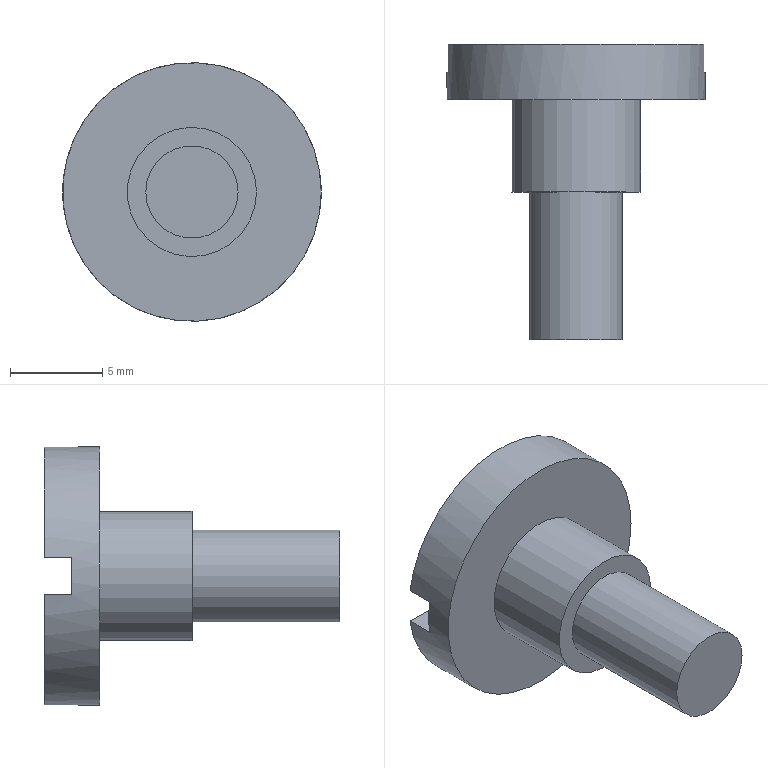Part | STEP file | 2-06.5 | 1 solid | 11 faces | box 14 x 16 x 14 mm | volume 769.46 mm3 | plane 8 | cylinder 3 | commonest cylinder face diameters 5 x1 7 x1 14 x1
STEP:
#1=CARTESIAN_POINT('',(0.,0.,0.));
#2=DIRECTION('',(0.,0.,1.));
#3=DIRECTION('',(1.,0.,0.));
#4=AXIS2_PLACEMENT_3D('',#1,#2,#3);
#5=CARTESIAN_POINT('',(3.5,0.,0.));
#6=VERTEX_POINT('',#5);
#7=CARTESIAN_POINT('',(0.,0.,0.));
#8=DIRECTION('',(0.,-1.,0.));
#9=DIRECTION('',(1.,0.,0.));
#10=AXIS2_PLACEMENT_3D('',#7,#8,#9);
#11=CIRCLE('',#10,3.5);
#12=CARTESIAN_POINT('',(0.,0.,0.));
#13=DIRECTION('',(0.,-1.,0.));
#14=DIRECTION('',(1.,0.,0.));
#15=AXIS2_PLACEMENT_3D('',#12,#13,#14);
#16=CYLINDRICAL_SURFACE('',#15,3.5);
#17=CARTESIAN_POINT('',(0.,0.));
#18=DIRECTION('',(1.,0.));
#19=VECTOR('',#18,1.);
#20=LINE('',#17,#19);
#21=(GEOMETRIC_REPRESENTATION_CONTEXT(2)PARAMETRIC_REPRESENTATION_CONTEXT()REPRESENTATION_CONTEXT('',''));
#22=DEFINITIONAL_REPRESENTATION('',(#20),#21);
#23=PCURVE('',#16,#22);
#24=CARTESIAN_POINT('',(-1.876,0.,0.));
#25=DIRECTION('',(0.,-1.,0.));
#26=DIRECTION('',(1.,0.,0.));
#27=AXIS2_PLACEMENT_3D('',#24,#25,#26);
#28=PLANE('',#27);
#29=CARTESIAN_POINT('',(1.876,0.));
#30=DIRECTION('',(1.,0.));
#31=AXIS2_PLACEMENT_2D('',#29,#30);
#32=CIRCLE('',#31,3.5);
#33=(GEOMETRIC_REPRESENTATION_CONTEXT(2)PARAMETRIC_REPRESENTATION_CONTEXT()REPRESENTATION_CONTEXT('',''));
#34=DEFINITIONAL_REPRESENTATION('',(#32),#33);
#35=PCURVE('',#28,#34);
#36=SURFACE_CURVE('',#11,(#23,#35),.PCURVE_S1.);
#37=EDGE_CURVE('',#6,#6,#36,.T.);
#38=ORIENTED_EDGE('',*,*,#37,.T.);
#39=CARTESIAN_POINT('',(3.5,-5.,0.));
#40=VERTEX_POINT('',#39);
#41=CARTESIAN_POINT('',(3.5,0.,0.));
#42=DIRECTION('',(0.,-1.,0.));
#43=VECTOR('',#42,1.);
#44=LINE('',#41,#43);
#45=CARTESIAN_POINT('',(6.283,0.));
#46=DIRECTION('',(0.,1.));
#47=VECTOR('',#46,1.);
#48=LINE('',#45,#47);
#49=(GEOMETRIC_REPRESENTATION_CONTEXT(2)PARAMETRIC_REPRESENTATION_CONTEXT()REPRESENTATION_CONTEXT('',''));
#50=DEFINITIONAL_REPRESENTATION('',(#48),#49);
#51=PCURVE('',#16,#50);
#52=CARTESIAN_POINT('',(0.,0.));
#53=DIRECTION('',(0.,1.));
#54=VECTOR('',#53,1.);
#55=LINE('',#52,#54);
#56=(GEOMETRIC_REPRESENTATION_CONTEXT(2)PARAMETRIC_REPRESENTATION_CONTEXT()REPRESENTATION_CONTEXT('',''));
#57=DEFINITIONAL_REPRESENTATION('',(#55),#56);
#58=PCURVE('',#16,#57);
#59=SEAM_CURVE('',#44,(#51,#58),.PCURVE_S1.);
#60=EDGE_CURVE('',#6,#40,#59,.T.);
#61=ORIENTED_EDGE('',*,*,#60,.T.);
#62=CARTESIAN_POINT('',(0.,-5.,0.));
#63=DIRECTION('',(0.,-1.,0.));
#64=DIRECTION('',(1.,0.,0.));
#65=AXIS2_PLACEMENT_3D('',#62,#63,#64);
#66=CIRCLE('',#65,3.5);
#67=CARTESIAN_POINT('',(0.,5.));
#68=DIRECTION('',(1.,0.));
#69=VECTOR('',#68,1.);
#70=LINE('',#67,#69);
#71=(GEOMETRIC_REPRESENTATION_CONTEXT(2)PARAMETRIC_REPRESENTATION_CONTEXT()REPRESENTATION_CONTEXT('',''));
#72=DEFINITIONAL_REPRESENTATION('',(#70),#71);
#73=PCURVE('',#16,#72);
#74=CARTESIAN_POINT('',(-0.9378,-5.,0.));
#75=DIRECTION('',(0.,-1.,0.));
#76=DIRECTION('',(1.,0.,0.));
#77=AXIS2_PLACEMENT_3D('',#74,#75,#76);
#78=PLANE('',#77);
#79=CARTESIAN_POINT('',(0.9378,0.));
#80=DIRECTION('',(1.,0.));
#81=AXIS2_PLACEMENT_2D('',#79,#80);
#82=CIRCLE('',#81,3.5);
#83=(GEOMETRIC_REPRESENTATION_CONTEXT(2)PARAMETRIC_REPRESENTATION_CONTEXT()REPRESENTATION_CONTEXT('',''));
#84=DEFINITIONAL_REPRESENTATION('',(#82),#83);
#85=PCURVE('',#78,#84);
#86=SURFACE_CURVE('',#66,(#73,#85),.PCURVE_S1.);
#87=EDGE_CURVE('',#40,#40,#86,.T.);
#88=ORIENTED_EDGE('',*,*,#87,.F.);
#89=ORIENTED_EDGE('',*,*,#60,.F.);
#90=EDGE_LOOP('',(#38,#61,#88,#89));
#91=FACE_BOUND('',#90,.T.);
#92=ADVANCED_FACE('',(#91),#16,.T.);
#93=CARTESIAN_POINT('',(7.,0.,0.));
#94=VERTEX_POINT('',#93);
#95=CARTESIAN_POINT('',(0.,0.,0.));
#96=DIRECTION('',(0.,-1.,0.));
#97=DIRECTION('',(1.,0.,0.));
#98=AXIS2_PLACEMENT_3D('',#95,#96,#97);
#99=CIRCLE('',#98,7.);
#100=CARTESIAN_POINT('',(1.876,0.));
#101=DIRECTION('',(1.,0.));
#102=AXIS2_PLACEMENT_2D('',#100,#101);
#103=CIRCLE('',#102,7.);
#104=(GEOMETRIC_REPRESENTATION_CONTEXT(2)PARAMETRIC_REPRESENTATION_CONTEXT()REPRESENTATION_CONTEXT('',''));
#105=DEFINITIONAL_REPRESENTATION('',(#103),#104);
#106=PCURVE('',#28,#105);
#107=CARTESIAN_POINT('',(0.,0.,0.));
#108=DIRECTION('',(0.,1.,0.));
#109=DIRECTION('',(1.,0.,0.));
#110=AXIS2_PLACEMENT_3D('',#107,#108,#109);
#111=CYLINDRICAL_SURFACE('',#110,7.);
#112=CARTESIAN_POINT('',(6.283,0.));
#113=DIRECTION('',(-1.,0.));
#114=VECTOR('',#113,1.);
#115=LINE('',#112,#114);
#116=(GEOMETRIC_REPRESENTATION_CONTEXT(2)PARAMETRIC_REPRESENTATION_CONTEXT()REPRESENTATION_CONTEXT('',''));
#117=DEFINITIONAL_REPRESENTATION('',(#115),#116);
#118=PCURVE('',#111,#117);
#119=SURFACE_CURVE('',#99,(#106,#118),.PCURVE_S1.);
#120=EDGE_CURVE('',#94,#94,#119,.T.);
#121=ORIENTED_EDGE('',*,*,#120,.T.);
#122=EDGE_LOOP('',(#121));
#123=FACE_BOUND('',#122,.T.);
#124=ORIENTED_EDGE('',*,*,#37,.F.);
#125=EDGE_LOOP('',(#124));
#126=FACE_BOUND('',#125,.T.);
#127=ADVANCED_FACE('',(#123,#126),#28,.T.);
#128=ORIENTED_EDGE('',*,*,#87,.T.);
#129=EDGE_LOOP('',(#128));
#130=FACE_BOUND('',#129,.T.);
#131=CARTESIAN_POINT('',(2.5,-5.,0.));
#132=VERTEX_POINT('',#131);
#133=CARTESIAN_POINT('',(0.,-5.,0.));
#134=DIRECTION('',(0.,-1.,0.));
#135=DIRECTION('',(1.,0.,0.));
#136=AXIS2_PLACEMENT_3D('',#133,#134,#135);
#137=CIRCLE('',#136,2.5);
#138=CARTESIAN_POINT('',(0.9378,0.));
#139=DIRECTION('',(1.,0.));
#140=AXIS2_PLACEMENT_2D('',#138,#139);
#141=CIRCLE('',#140,2.5);
#142=(GEOMETRIC_REPRESENTATION_CONTEXT(2)PARAMETRIC_REPRESENTATION_CONTEXT()REPRESENTATION_CONTEXT('',''));
#143=DEFINITIONAL_REPRESENTATION('',(#141),#142);
#144=PCURVE('',#78,#143);
#145=CARTESIAN_POINT('',(0.,-5.,0.));
#146=DIRECTION('',(0.,-1.,0.));
#147=DIRECTION('',(1.,0.,0.));
#148=AXIS2_PLACEMENT_3D('',#145,#146,#147);
#149=CYLINDRICAL_SURFACE('',#148,2.5);
#150=CARTESIAN_POINT('',(0.,0.));
#151=DIRECTION('',(1.,0.));
#152=VECTOR('',#151,1.);
#153=LINE('',#150,#152);
#154=(GEOMETRIC_REPRESENTATION_CONTEXT(2)PARAMETRIC_REPRESENTATION_CONTEXT()REPRESENTATION_CONTEXT('',''));
#155=DEFINITIONAL_REPRESENTATION('',(#153),#154);
#156=PCURVE('',#149,#155);
#157=SURFACE_CURVE('',#137,(#144,#156),.PCURVE_S1.);
#158=EDGE_CURVE('',#132,#132,#157,.T.);
#159=ORIENTED_EDGE('',*,*,#158,.F.);
#160=EDGE_LOOP('',(#159));
#161=FACE_BOUND('',#160,.T.);
#162=ADVANCED_FACE('',(#130,#161),#78,.T.);
#163=ORIENTED_EDGE('',*,*,#158,.T.);
#164=CARTESIAN_POINT('',(2.5,-13.,0.));
#165=VERTEX_POINT('',#164);
#166=CARTESIAN_POINT('',(2.5,-5.,0.));
#167=DIRECTION('',(0.,-1.,0.));
#168=VECTOR('',#167,1.);
#169=LINE('',#166,#168);
#170=CARTESIAN_POINT('',(6.283,0.));
#171=DIRECTION('',(0.,1.));
#172=VECTOR('',#171,1.);
#173=LINE('',#170,#172);
#174=(GEOMETRIC_REPRESENTATION_CONTEXT(2)PARAMETRIC_REPRESENTATION_CONTEXT()REPRESENTATION_CONTEXT('',''));
#175=DEFINITIONAL_REPRESENTATION('',(#173),#174);
#176=PCURVE('',#149,#175);
#177=CARTESIAN_POINT('',(0.,0.));
#178=DIRECTION('',(0.,1.));
#179=VECTOR('',#178,1.);
#180=LINE('',#177,#179);
#181=(GEOMETRIC_REPRESENTATION_CONTEXT(2)PARAMETRIC_REPRESENTATION_CONTEXT()REPRESENTATION_CONTEXT('',''));
#182=DEFINITIONAL_REPRESENTATION('',(#180),#181);
#183=PCURVE('',#149,#182);
#184=SEAM_CURVE('',#169,(#176,#183),.PCURVE_S1.);
#185=EDGE_CURVE('',#132,#165,#184,.T.);
#186=ORIENTED_EDGE('',*,*,#185,.T.);
#187=CARTESIAN_POINT('',(0.,-13.,0.));
#188=DIRECTION('',(0.,-1.,0.));
#189=DIRECTION('',(1.,0.,0.));
#190=AXIS2_PLACEMENT_3D('',#187,#188,#189);
#191=CIRCLE('',#190,2.5);
#192=CARTESIAN_POINT('',(0.,8.));
#193=DIRECTION('',(1.,0.));
#194=VECTOR('',#193,1.);
#195=LINE('',#192,#194);
#196=(GEOMETRIC_REPRESENTATION_CONTEXT(2)PARAMETRIC_REPRESENTATION_CONTEXT()REPRESENTATION_CONTEXT('',''));
#197=DEFINITIONAL_REPRESENTATION('',(#195),#196);
#198=PCURVE('',#149,#197);
#199=CARTESIAN_POINT('',(-0.6699,-13.,0.));
#200=DIRECTION('',(0.,-1.,0.));
#201=DIRECTION('',(1.,0.,0.));
#202=AXIS2_PLACEMENT_3D('',#199,#200,#201);
#203=PLANE('',#202);
#204=CARTESIAN_POINT('',(0.6699,0.));
#205=DIRECTION('',(1.,0.));
#206=AXIS2_PLACEMENT_2D('',#204,#205);
#207=CIRCLE('',#206,2.5);
#208=(GEOMETRIC_REPRESENTATION_CONTEXT(2)PARAMETRIC_REPRESENTATION_CONTEXT()REPRESENTATION_CONTEXT('',''));
#209=DEFINITIONAL_REPRESENTATION('',(#207),#208);
#210=PCURVE('',#203,#209);
#211=SURFACE_CURVE('',#191,(#198,#210),.PCURVE_S1.);
#212=EDGE_CURVE('',#165,#165,#211,.T.);
#213=ORIENTED_EDGE('',*,*,#212,.F.);
#214=ORIENTED_EDGE('',*,*,#185,.F.);
#215=EDGE_LOOP('',(#163,#186,#213,#214));
#216=FACE_BOUND('',#215,.T.);
#217=ADVANCED_FACE('',(#216),#149,.T.);
#218=ORIENTED_EDGE('',*,*,#212,.T.);
#219=EDGE_LOOP('',(#218));
#220=FACE_BOUND('',#219,.T.);
#221=ADVANCED_FACE('',(#220),#203,.T.);
#222=CARTESIAN_POINT('',(7.,1.5,0.));
#223=VERTEX_POINT('',#222);
#224=CARTESIAN_POINT('',(7.,0.,0.));
#225=DIRECTION('',(0.,1.,0.));
#226=VECTOR('',#225,1.);
#227=LINE('',#224,#226);
#228=CARTESIAN_POINT('',(6.283,0.));
#229=DIRECTION('',(0.,1.));
#230=VECTOR('',#229,1.);
#231=LINE('',#228,#230);
#232=(GEOMETRIC_REPRESENTATION_CONTEXT(2)PARAMETRIC_REPRESENTATION_CONTEXT()REPRESENTATION_CONTEXT('',''));
#233=DEFINITIONAL_REPRESENTATION('',(#231),#232);
#234=PCURVE('',#111,#233);
#235=CARTESIAN_POINT('',(0.,0.));
#236=DIRECTION('',(0.,1.));
#237=VECTOR('',#236,1.);
#238=LINE('',#235,#237);
#239=(GEOMETRIC_REPRESENTATION_CONTEXT(2)PARAMETRIC_REPRESENTATION_CONTEXT()REPRESENTATION_CONTEXT('',''));
#240=DEFINITIONAL_REPRESENTATION('',(#238),#239);
#241=PCURVE('',#111,#240);
#242=SEAM_CURVE('',#227,(#234,#241),.PCURVE_S1.);
#243=EDGE_CURVE('',#94,#223,#242,.T.);
#244=ORIENTED_EDGE('',*,*,#243,.T.);
#245=CARTESIAN_POINT('',(6.928,1.5,1.));
#246=VERTEX_POINT('',#245);
#247=CARTESIAN_POINT('',(0.,1.5,0.));
#248=DIRECTION('',(0.,1.,0.));
#249=DIRECTION('',(0.9897,0.,0.1429));
#250=AXIS2_PLACEMENT_3D('',#247,#248,#249);
#251=CIRCLE('',#250,7.);
#252=CARTESIAN_POINT('',(6.14,1.5));
#253=DIRECTION('',(1.,0.));
#254=VECTOR('',#253,1.);
#255=LINE('',#252,#254);
#256=(GEOMETRIC_REPRESENTATION_CONTEXT(2)PARAMETRIC_REPRESENTATION_CONTEXT()REPRESENTATION_CONTEXT('',''));
#257=DEFINITIONAL_REPRESENTATION('',(#255),#256);
#258=PCURVE('',#111,#257);
#259=CARTESIAN_POINT('',(0.,1.5,0.));
#260=DIRECTION('',(0.,-1.,0.));
#261=DIRECTION('',(0.,0.,-1.));
#262=AXIS2_PLACEMENT_3D('',#259,#260,#261);
#263=PLANE('',#262);
#264=CARTESIAN_POINT('',(-1.,6.928));
#265=CARTESIAN_POINT('',(11.,8.66));
#266=CARTESIAN_POINT('',(6.5,-2.598));
#267=CARTESIAN_POINT('',(2.,-13.856));
#268=CARTESIAN_POINT('',(-5.5,-4.33));
#269=CARTESIAN_POINT('',(-13.,5.196));
#270=CARTESIAN_POINT('',(-1.,6.928));
#271=(BOUNDED_CURVE()B_SPLINE_CURVE(2,(#264,#265,#266,#267,#268,#269,#270),.UNSPECIFIED.,.T.,.F.)B_SPLINE_CURVE_WITH_KNOTS((1,2,2,2,2,1),(-2.094,0.,2.094,4.189,6.283,8.378),.UNSPECIFIED.)CURVE()GEOMETRIC_REPRESENTATION_ITEM()RATIONAL_B_SPLINE_CURVE((1.,0.5,1.,0.5,1.,0.5,1.))REPRESENTATION_ITEM(''));
#272=(GEOMETRIC_REPRESENTATION_CONTEXT(2)PARAMETRIC_REPRESENTATION_CONTEXT()REPRESENTATION_CONTEXT('',''));
#273=DEFINITIONAL_REPRESENTATION('',(#271),#272);
#274=PCURVE('',#263,#273);
#275=SURFACE_CURVE('',#251,(#258,#274),.PCURVE_S1.);
#276=EDGE_CURVE('',#246,#223,#275,.T.);
#277=ORIENTED_EDGE('',*,*,#276,.F.);
#278=CARTESIAN_POINT('',(6.928,3.,1.));
#279=VERTEX_POINT('',#278);
#280=CARTESIAN_POINT('',(6.928,3.,1.));
#281=DIRECTION('',(0.,-1.,0.));
#282=VECTOR('',#281,1.);
#283=LINE('',#280,#282);
#284=CARTESIAN_POINT('',(6.14,3.));
#285=DIRECTION('',(0.,-1.));
#286=VECTOR('',#285,1.);
#287=LINE('',#284,#286);
#288=(GEOMETRIC_REPRESENTATION_CONTEXT(2)PARAMETRIC_REPRESENTATION_CONTEXT()REPRESENTATION_CONTEXT('',''));
#289=DEFINITIONAL_REPRESENTATION('',(#287),#288);
#290=PCURVE('',#111,#289);
#291=CARTESIAN_POINT('',(0.,3.,1.));
#292=DIRECTION('',(0.,0.,1.));
#293=DIRECTION('',(0.,-1.,0.));
#294=AXIS2_PLACEMENT_3D('',#291,#292,#293);
#295=PLANE('',#294);
#296=CARTESIAN_POINT('',(0.,6.928));
#297=DIRECTION('',(1.,0.));
#298=VECTOR('',#297,1.);
#299=LINE('',#296,#298);
#300=(GEOMETRIC_REPRESENTATION_CONTEXT(2)PARAMETRIC_REPRESENTATION_CONTEXT()REPRESENTATION_CONTEXT('',''));
#301=DEFINITIONAL_REPRESENTATION('',(#299),#300);
#302=PCURVE('',#295,#301);
#303=SURFACE_CURVE('',#283,(#290,#302),.PCURVE_S1.);
#304=EDGE_CURVE('',#279,#246,#303,.T.);
#305=ORIENTED_EDGE('',*,*,#304,.F.);
#306=CARTESIAN_POINT('',(-6.928,3.,1.));
#307=VERTEX_POINT('',#306);
#308=CARTESIAN_POINT('',(0.,3.,0.));
#309=DIRECTION('',(0.,-1.,0.));
#310=DIRECTION('',(0.9897,0.,0.1429));
#311=AXIS2_PLACEMENT_3D('',#308,#309,#310);
#312=CIRCLE('',#311,7.);
#313=CARTESIAN_POINT('',(6.14,3.));
#314=DIRECTION('',(-1.,0.));
#315=VECTOR('',#314,1.);
#316=LINE('',#313,#315);
#317=(GEOMETRIC_REPRESENTATION_CONTEXT(2)PARAMETRIC_REPRESENTATION_CONTEXT()REPRESENTATION_CONTEXT('',''));
#318=DEFINITIONAL_REPRESENTATION('',(#316),#317);
#319=PCURVE('',#111,#318);
#320=CARTESIAN_POINT('',(0.,3.,0.));
#321=DIRECTION('',(0.,-1.,0.));
#322=DIRECTION('',(1.,0.,0.));
#323=AXIS2_PLACEMENT_3D('',#320,#321,#322);
#324=PLANE('',#323);
#325=CARTESIAN_POINT('',(0.,0.));
#326=DIRECTION('',(0.9897,0.1429));
#327=AXIS2_PLACEMENT_2D('',#325,#326);
#328=CIRCLE('',#327,7.);
#329=(GEOMETRIC_REPRESENTATION_CONTEXT(2)PARAMETRIC_REPRESENTATION_CONTEXT()REPRESENTATION_CONTEXT('',''));
#330=DEFINITIONAL_REPRESENTATION('',(#328),#329);
#331=PCURVE('',#324,#330);
#332=SURFACE_CURVE('',#312,(#319,#331),.PCURVE_S1.);
#333=EDGE_CURVE('',#279,#307,#332,.T.);
#334=ORIENTED_EDGE('',*,*,#333,.T.);
#335=CARTESIAN_POINT('',(-6.928,1.5,1.));
#336=VERTEX_POINT('',#335);
#337=CARTESIAN_POINT('',(-6.928,1.5,1.));
#338=DIRECTION('',(0.,1.,0.));
#339=VECTOR('',#338,1.);
#340=LINE('',#337,#339);
#341=CARTESIAN_POINT('',(3.285,1.5));
#342=DIRECTION('',(0.,1.));
#343=VECTOR('',#342,1.);
#344=LINE('',#341,#343);
#345=(GEOMETRIC_REPRESENTATION_CONTEXT(2)PARAMETRIC_REPRESENTATION_CONTEXT()REPRESENTATION_CONTEXT('',''));
#346=DEFINITIONAL_REPRESENTATION('',(#344),#345);
#347=PCURVE('',#111,#346);
#348=CARTESIAN_POINT('',(1.5,-6.928));
#349=DIRECTION('',(-1.,0.));
#350=VECTOR('',#349,1.);
#351=LINE('',#348,#350);
#352=(GEOMETRIC_REPRESENTATION_CONTEXT(2)PARAMETRIC_REPRESENTATION_CONTEXT()REPRESENTATION_CONTEXT('',''));
#353=DEFINITIONAL_REPRESENTATION('',(#351),#352);
#354=PCURVE('',#295,#353);
#355=SURFACE_CURVE('',#340,(#347,#354),.PCURVE_S1.);
#356=EDGE_CURVE('',#336,#307,#355,.T.);
#357=ORIENTED_EDGE('',*,*,#356,.F.);
#358=CARTESIAN_POINT('',(-6.928,1.5,-1.));
#359=VERTEX_POINT('',#358);
#360=CARTESIAN_POINT('',(0.,1.5,0.));
#361=DIRECTION('',(0.,1.,0.));
#362=DIRECTION('',(-0.9897,0.,-0.1429));
#363=AXIS2_PLACEMENT_3D('',#360,#361,#362);
#364=CIRCLE('',#363,7.);
#365=CARTESIAN_POINT('',(2.998,1.5));
#366=DIRECTION('',(1.,0.));
#367=VECTOR('',#366,1.);
#368=LINE('',#365,#367);
#369=(GEOMETRIC_REPRESENTATION_CONTEXT(2)PARAMETRIC_REPRESENTATION_CONTEXT()REPRESENTATION_CONTEXT('',''));
#370=DEFINITIONAL_REPRESENTATION('',(#368),#369);
#371=PCURVE('',#111,#370);
#372=CARTESIAN_POINT('',(1.,-6.928));
#373=CARTESIAN_POINT('',(-11.,-8.66));
#374=CARTESIAN_POINT('',(-6.5,2.598));
#375=CARTESIAN_POINT('',(-2.,13.856));
#376=CARTESIAN_POINT('',(5.5,4.33));
#377=CARTESIAN_POINT('',(13.,-5.196));
#378=CARTESIAN_POINT('',(1.,-6.928));
#379=(BOUNDED_CURVE()B_SPLINE_CURVE(2,(#372,#373,#374,#375,#376,#377,#378),.UNSPECIFIED.,.T.,.F.)B_SPLINE_CURVE_WITH_KNOTS((1,2,2,2,2,1),(-2.094,0.,2.094,4.189,6.283,8.378),.UNSPECIFIED.)CURVE()GEOMETRIC_REPRESENTATION_ITEM()RATIONAL_B_SPLINE_CURVE((1.,0.5,1.,0.5,1.,0.5,1.))REPRESENTATION_ITEM(''));
#380=(GEOMETRIC_REPRESENTATION_CONTEXT(2)PARAMETRIC_REPRESENTATION_CONTEXT()REPRESENTATION_CONTEXT('',''));
#381=DEFINITIONAL_REPRESENTATION('',(#379),#380);
#382=PCURVE('',#263,#381);
#383=SURFACE_CURVE('',#364,(#371,#382),.PCURVE_S1.);
#384=EDGE_CURVE('',#359,#336,#383,.T.);
#385=ORIENTED_EDGE('',*,*,#384,.F.);
#386=CARTESIAN_POINT('',(-6.928,3.,-1.));
#387=VERTEX_POINT('',#386);
#388=CARTESIAN_POINT('',(-6.928,3.,-1.));
#389=DIRECTION('',(0.,-1.,0.));
#390=VECTOR('',#389,1.);
#391=LINE('',#388,#390);
#392=CARTESIAN_POINT('',(2.998,3.));
#393=DIRECTION('',(0.,-1.));
#394=VECTOR('',#393,1.);
#395=LINE('',#392,#394);
#396=(GEOMETRIC_REPRESENTATION_CONTEXT(2)PARAMETRIC_REPRESENTATION_CONTEXT()REPRESENTATION_CONTEXT('',''));
#397=DEFINITIONAL_REPRESENTATION('',(#395),#396);
#398=PCURVE('',#111,#397);
#399=CARTESIAN_POINT('',(0.,3.,-1.));
#400=DIRECTION('',(0.,0.,-1.));
#401=DIRECTION('',(0.,1.,0.));
#402=AXIS2_PLACEMENT_3D('',#399,#400,#401);
#403=PLANE('',#402);
#404=CARTESIAN_POINT('',(0.,-6.928));
#405=DIRECTION('',(-1.,0.));
#406=VECTOR('',#405,1.);
#407=LINE('',#404,#406);
#408=(GEOMETRIC_REPRESENTATION_CONTEXT(2)PARAMETRIC_REPRESENTATION_CONTEXT()REPRESENTATION_CONTEXT('',''));
#409=DEFINITIONAL_REPRESENTATION('',(#407),#408);
#410=PCURVE('',#403,#409);
#411=SURFACE_CURVE('',#391,(#398,#410),.PCURVE_S1.);
#412=EDGE_CURVE('',#387,#359,#411,.T.);
#413=ORIENTED_EDGE('',*,*,#412,.F.);
#414=CARTESIAN_POINT('',(6.928,3.,-1.));
#415=VERTEX_POINT('',#414);
#416=CARTESIAN_POINT('',(0.,3.,0.));
#417=DIRECTION('',(0.,-1.,0.));
#418=DIRECTION('',(-0.9897,0.,-0.1429));
#419=AXIS2_PLACEMENT_3D('',#416,#417,#418);
#420=CIRCLE('',#419,7.);
#421=CARTESIAN_POINT('',(2.998,3.));
#422=DIRECTION('',(-1.,0.));
#423=VECTOR('',#422,1.);
#424=LINE('',#421,#423);
#425=(GEOMETRIC_REPRESENTATION_CONTEXT(2)PARAMETRIC_REPRESENTATION_CONTEXT()REPRESENTATION_CONTEXT('',''));
#426=DEFINITIONAL_REPRESENTATION('',(#424),#425);
#427=PCURVE('',#111,#426);
#428=CARTESIAN_POINT('',(0.,3.,0.));
#429=DIRECTION('',(0.,-1.,0.));
#430=DIRECTION('',(1.,0.,0.));
#431=AXIS2_PLACEMENT_3D('',#428,#429,#430);
#432=PLANE('',#431);
#433=CARTESIAN_POINT('',(0.,0.));
#434=DIRECTION('',(-0.9897,-0.1429));
#435=AXIS2_PLACEMENT_2D('',#433,#434);
#436=CIRCLE('',#435,7.);
#437=(GEOMETRIC_REPRESENTATION_CONTEXT(2)PARAMETRIC_REPRESENTATION_CONTEXT()REPRESENTATION_CONTEXT('',''));
#438=DEFINITIONAL_REPRESENTATION('',(#436),#437);
#439=PCURVE('',#432,#438);
#440=SURFACE_CURVE('',#420,(#427,#439),.PCURVE_S1.);
#441=EDGE_CURVE('',#387,#415,#440,.T.);
#442=ORIENTED_EDGE('',*,*,#441,.T.);
#443=CARTESIAN_POINT('',(6.928,1.5,-1.));
#444=VERTEX_POINT('',#443);
#445=CARTESIAN_POINT('',(6.928,1.5,-1.));
#446=DIRECTION('',(0.,1.,0.));
#447=VECTOR('',#446,1.);
#448=LINE('',#445,#447);
#449=CARTESIAN_POINT('',(0.1433,1.5));
#450=DIRECTION('',(0.,1.));
#451=VECTOR('',#450,1.);
#452=LINE('',#449,#451);
#453=(GEOMETRIC_REPRESENTATION_CONTEXT(2)PARAMETRIC_REPRESENTATION_CONTEXT()REPRESENTATION_CONTEXT('',''));
#454=DEFINITIONAL_REPRESENTATION('',(#452),#453);
#455=PCURVE('',#111,#454);
#456=CARTESIAN_POINT('',(-1.5,6.928));
#457=DIRECTION('',(1.,0.));
#458=VECTOR('',#457,1.);
#459=LINE('',#456,#458);
#460=(GEOMETRIC_REPRESENTATION_CONTEXT(2)PARAMETRIC_REPRESENTATION_CONTEXT()REPRESENTATION_CONTEXT('',''));
#461=DEFINITIONAL_REPRESENTATION('',(#459),#460);
#462=PCURVE('',#403,#461);
#463=SURFACE_CURVE('',#448,(#455,#462),.PCURVE_S1.);
#464=EDGE_CURVE('',#444,#415,#463,.T.);
#465=ORIENTED_EDGE('',*,*,#464,.F.);
#466=CARTESIAN_POINT('',(0.,1.5,0.));
#467=DIRECTION('',(0.,1.,0.));
#468=DIRECTION('',(1.,0.,0.));
#469=AXIS2_PLACEMENT_3D('',#466,#467,#468);
#470=CIRCLE('',#469,7.);
#471=CARTESIAN_POINT('',(0.,1.5));
#472=DIRECTION('',(1.,0.));
#473=VECTOR('',#472,1.);
#474=LINE('',#471,#473);
#475=(GEOMETRIC_REPRESENTATION_CONTEXT(2)PARAMETRIC_REPRESENTATION_CONTEXT()REPRESENTATION_CONTEXT('',''));
#476=DEFINITIONAL_REPRESENTATION('',(#474),#475);
#477=PCURVE('',#111,#476);
#478=CARTESIAN_POINT('',(0.,7.));
#479=CARTESIAN_POINT('',(12.124,7.));
#480=CARTESIAN_POINT('',(6.062,-3.5));
#481=CARTESIAN_POINT('',(0.,-14.));
#482=CARTESIAN_POINT('',(-6.062,-3.5));
#483=CARTESIAN_POINT('',(-12.124,7.));
#484=CARTESIAN_POINT('',(0.,7.));
#485=(BOUNDED_CURVE()B_SPLINE_CURVE(2,(#478,#479,#480,#481,#482,#483,#484),.UNSPECIFIED.,.T.,.F.)B_SPLINE_CURVE_WITH_KNOTS((1,2,2,2,2,1),(-2.094,0.,2.094,4.189,6.283,8.378),.UNSPECIFIED.)CURVE()GEOMETRIC_REPRESENTATION_ITEM()RATIONAL_B_SPLINE_CURVE((1.,0.5,1.,0.5,1.,0.5,1.))REPRESENTATION_ITEM(''));
#486=(GEOMETRIC_REPRESENTATION_CONTEXT(2)PARAMETRIC_REPRESENTATION_CONTEXT()REPRESENTATION_CONTEXT('',''));
#487=DEFINITIONAL_REPRESENTATION('',(#485),#486);
#488=PCURVE('',#263,#487);
#489=SURFACE_CURVE('',#470,(#477,#488),.PCURVE_S1.);
#490=EDGE_CURVE('',#223,#444,#489,.T.);
#491=ORIENTED_EDGE('',*,*,#490,.F.);
#492=ORIENTED_EDGE('',*,*,#243,.F.);
#493=ORIENTED_EDGE('',*,*,#120,.F.);
#494=EDGE_LOOP('',(#244,#277,#305,#334,#357,#385,#413,#442,#465,#491,#492,#493));
#495=FACE_BOUND('',#494,.T.);
#496=ADVANCED_FACE('',(#495),#111,.T.);
#497=ORIENTED_EDGE('',*,*,#441,.T.);
#498=CARTESIAN_POINT('',(6.928,3.,-1.));
#499=DIRECTION('',(-1.,0.,0.));
#500=VECTOR('',#499,1.);
#501=LINE('',#498,#500);
#502=CARTESIAN_POINT('',(6.928,-1.));
#503=DIRECTION('',(-1.,0.));
#504=VECTOR('',#503,1.);
#505=LINE('',#502,#504);
#506=(GEOMETRIC_REPRESENTATION_CONTEXT(2)PARAMETRIC_REPRESENTATION_CONTEXT()REPRESENTATION_CONTEXT('',''));
#507=DEFINITIONAL_REPRESENTATION('',(#505),#506);
#508=PCURVE('',#432,#507);
#509=CARTESIAN_POINT('',(0.,6.928));
#510=DIRECTION('',(0.,-1.));
#511=VECTOR('',#510,1.);
#512=LINE('',#509,#511);
#513=(GEOMETRIC_REPRESENTATION_CONTEXT(2)PARAMETRIC_REPRESENTATION_CONTEXT()REPRESENTATION_CONTEXT('',''));
#514=DEFINITIONAL_REPRESENTATION('',(#512),#513);
#515=PCURVE('',#403,#514);
#516=SURFACE_CURVE('',#501,(#508,#515),.PCURVE_S1.);
#517=EDGE_CURVE('',#415,#387,#516,.T.);
#518=ORIENTED_EDGE('',*,*,#517,.T.);
#519=EDGE_LOOP('',(#497,#518));
#520=FACE_BOUND('',#519,.F.);
#521=ADVANCED_FACE('',(#520),#432,.F.);
#522=ORIENTED_EDGE('',*,*,#333,.T.);
#523=CARTESIAN_POINT('',(-6.928,3.,1.));
#524=DIRECTION('',(1.,0.,0.));
#525=VECTOR('',#524,1.);
#526=LINE('',#523,#525);
#527=CARTESIAN_POINT('',(-6.928,1.));
#528=DIRECTION('',(1.,0.));
#529=VECTOR('',#528,1.);
#530=LINE('',#527,#529);
#531=(GEOMETRIC_REPRESENTATION_CONTEXT(2)PARAMETRIC_REPRESENTATION_CONTEXT()REPRESENTATION_CONTEXT('',''));
#532=DEFINITIONAL_REPRESENTATION('',(#530),#531);
#533=PCURVE('',#324,#532);
#534=CARTESIAN_POINT('',(0.,-6.928));
#535=DIRECTION('',(0.,1.));
#536=VECTOR('',#535,1.);
#537=LINE('',#534,#536);
#538=(GEOMETRIC_REPRESENTATION_CONTEXT(2)PARAMETRIC_REPRESENTATION_CONTEXT()REPRESENTATION_CONTEXT('',''));
#539=DEFINITIONAL_REPRESENTATION('',(#537),#538);
#540=PCURVE('',#295,#539);
#541=SURFACE_CURVE('',#526,(#533,#540),.PCURVE_S1.);
#542=EDGE_CURVE('',#307,#279,#541,.T.);
#543=ORIENTED_EDGE('',*,*,#542,.T.);
#544=EDGE_LOOP('',(#522,#543));
#545=FACE_BOUND('',#544,.F.);
#546=ADVANCED_FACE('',(#545),#324,.F.);
#547=CARTESIAN_POINT('',(-6.928,1.5,1.));
#548=DIRECTION('',(1.,0.,0.));
#549=VECTOR('',#548,1.);
#550=LINE('',#547,#549);
#551=CARTESIAN_POINT('',(-1.,-6.928));
#552=DIRECTION('',(0.,1.));
#553=VECTOR('',#552,1.);
#554=LINE('',#551,#553);
#555=(GEOMETRIC_REPRESENTATION_CONTEXT(2)PARAMETRIC_REPRESENTATION_CONTEXT()REPRESENTATION_CONTEXT('',''));
#556=DEFINITIONAL_REPRESENTATION('',(#554),#555);
#557=PCURVE('',#263,#556);
#558=CARTESIAN_POINT('',(1.5,-6.928));
#559=DIRECTION('',(0.,1.));
#560=VECTOR('',#559,1.);
#561=LINE('',#558,#560);
#562=(GEOMETRIC_REPRESENTATION_CONTEXT(2)PARAMETRIC_REPRESENTATION_CONTEXT()REPRESENTATION_CONTEXT('',''));
#563=DEFINITIONAL_REPRESENTATION('',(#561),#562);
#564=PCURVE('',#295,#563);
#565=SURFACE_CURVE('',#550,(#557,#564),.PCURVE_S1.);
#566=EDGE_CURVE('',#336,#246,#565,.T.);
#567=ORIENTED_EDGE('',*,*,#566,.F.);
#568=ORIENTED_EDGE('',*,*,#384,.F.);
#569=CARTESIAN_POINT('',(-6.928,1.5,-1.));
#570=DIRECTION('',(1.,0.,0.));
#571=VECTOR('',#570,1.);
#572=LINE('',#569,#571);
#573=CARTESIAN_POINT('',(1.,-6.928));
#574=DIRECTION('',(0.,1.));
#575=VECTOR('',#574,1.);
#576=LINE('',#573,#575);
#577=(GEOMETRIC_REPRESENTATION_CONTEXT(2)PARAMETRIC_REPRESENTATION_CONTEXT()REPRESENTATION_CONTEXT('',''));
#578=DEFINITIONAL_REPRESENTATION('',(#576),#577);
#579=PCURVE('',#263,#578);
#580=CARTESIAN_POINT('',(-1.5,-6.928));
#581=DIRECTION('',(0.,1.));
#582=VECTOR('',#581,1.);
#583=LINE('',#580,#582);
#584=(GEOMETRIC_REPRESENTATION_CONTEXT(2)PARAMETRIC_REPRESENTATION_CONTEXT()REPRESENTATION_CONTEXT('',''));
#585=DEFINITIONAL_REPRESENTATION('',(#583),#584);
#586=PCURVE('',#403,#585);
#587=SURFACE_CURVE('',#572,(#579,#586),.PCURVE_S1.);
#588=EDGE_CURVE('',#359,#444,#587,.T.);
#589=ORIENTED_EDGE('',*,*,#588,.T.);
#590=ORIENTED_EDGE('',*,*,#490,.F.);
#591=ORIENTED_EDGE('',*,*,#276,.F.);
#592=EDGE_LOOP('',(#567,#568,#589,#590,#591));
#593=FACE_BOUND('',#592,.F.);
#594=ADVANCED_FACE('',(#593),#263,.F.);
#595=ORIENTED_EDGE('',*,*,#588,.F.);
#596=ORIENTED_EDGE('',*,*,#412,.F.);
#597=ORIENTED_EDGE('',*,*,#517,.F.);
#598=ORIENTED_EDGE('',*,*,#464,.F.);
#599=EDGE_LOOP('',(#595,#596,#597,#598));
#600=FACE_BOUND('',#599,.F.);
#601=ADVANCED_FACE('',(#600),#403,.F.);
#602=ORIENTED_EDGE('',*,*,#566,.T.);
#603=ORIENTED_EDGE('',*,*,#304,.F.);
#604=ORIENTED_EDGE('',*,*,#542,.F.);
#605=ORIENTED_EDGE('',*,*,#356,.F.);
#606=EDGE_LOOP('',(#602,#603,#604,#605));
#607=FACE_BOUND('',#606,.F.);
#608=ADVANCED_FACE('',(#607),#295,.F.);
#609=CLOSED_SHELL('',(#92,#127,#162,#217,#221,#496,#521,#546,#594,#601,#608));
#610=MANIFOLD_SOLID_BREP('',#609);
#611=(LENGTH_UNIT()NAMED_UNIT(*)SI_UNIT(.MILLI.,.METRE.));
#612=UNCERTAINTY_MEASURE_WITH_UNIT(LENGTH_MEASURE(0.0000001),#611,'','');
#613=(NAMED_UNIT(*)PLANE_ANGLE_UNIT()SI_UNIT($,.RADIAN.));
#614=(NAMED_UNIT(*)SI_UNIT($,.STERADIAN.)SOLID_ANGLE_UNIT());
#615=(GEOMETRIC_REPRESENTATION_CONTEXT(3)GLOBAL_UNCERTAINTY_ASSIGNED_CONTEXT((#612))GLOBAL_UNIT_ASSIGNED_CONTEXT((#611,#613,#614))REPRESENTATION_CONTEXT('',''));
#616=ADVANCED_BREP_SHAPE_REPRESENTATION('',(#4,#610),#615);